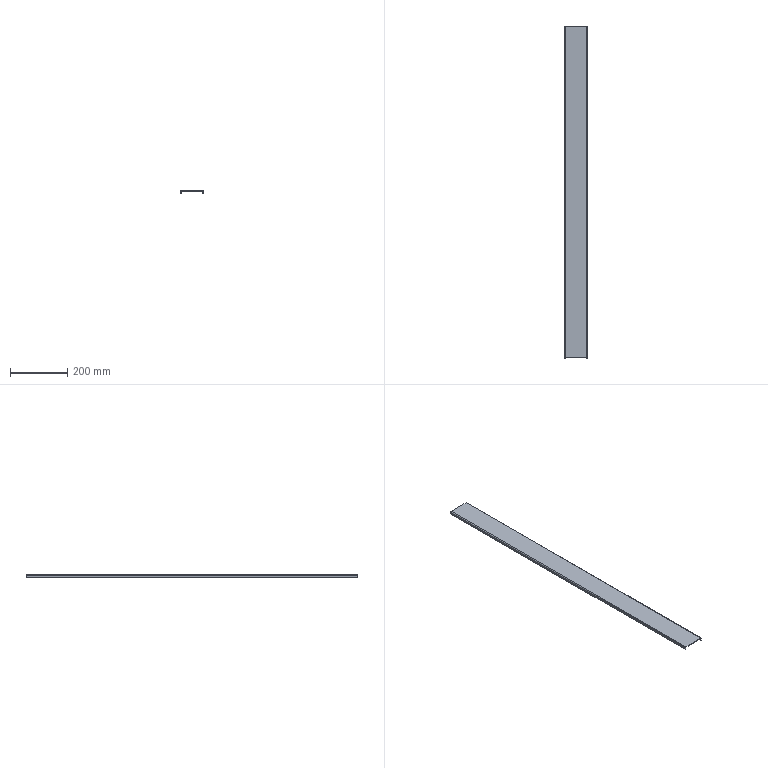Part | SolidWorks | features BaseBody 1 | 1 solid | 22 faces | box 80 x 1161 x 10 mm | volume 271377 mm3 | plane 18 | cylinder 4 | commonest cylinder face diameters 1 x2 6 x2
STEP:
#1=CARTESIAN_POINT('',(-37.5,580.5,-10.));
#2=VERTEX_POINT('',#1);
#3=CARTESIAN_POINT('',(-37.5,-580.5,-10.));
#4=VERTEX_POINT('',#3);
#5=CARTESIAN_POINT('',(-37.5,-580.5,-10.));
#6=DIRECTION('',(0.,-1.,0.));
#7=VECTOR('',#6,1000.);
#8=LINE('',#5,#7);
#9=EDGE_CURVE('',#2,#4,#8,.T.);
#10=ORIENTED_EDGE('',*,*,#9,.T.);
#11=CARTESIAN_POINT('',(-40.,-580.5,-10.));
#12=VERTEX_POINT('',#11);
#13=CARTESIAN_POINT('',(-40.,-580.5,-10.));
#14=DIRECTION('',(1.,0.,0.));
#15=VECTOR('',#14,1000.);
#16=LINE('',#13,#15);
#17=EDGE_CURVE('',#12,#4,#16,.T.);
#18=ORIENTED_EDGE('',*,*,#17,.F.);
#19=CARTESIAN_POINT('',(-40.,580.5,-10.));
#20=VERTEX_POINT('',#19);
#21=CARTESIAN_POINT('',(-40.,0.,-10.));
#22=DIRECTION('',(0.,-1.,0.));
#23=VECTOR('',#22,1000.);
#24=LINE('',#21,#23);
#25=EDGE_CURVE('',#20,#12,#24,.T.);
#26=ORIENTED_EDGE('',*,*,#25,.F.);
#27=CARTESIAN_POINT('',(-40.,580.5,-10.));
#28=DIRECTION('',(1.,0.,0.));
#29=VECTOR('',#28,1000.);
#30=LINE('',#27,#29);
#31=EDGE_CURVE('',#20,#2,#30,.T.);
#32=ORIENTED_EDGE('',*,*,#31,.T.);
#33=EDGE_LOOP('',(#10,#18,#26,#32));
#34=FACE_OUTER_BOUND('',#33,.T.);
#35=CARTESIAN_POINT('',(-40.,-580.5,-10.));
#36=DIRECTION('',(0.,0.,1.));
#37=DIRECTION('',(1.,0.,0.));
#38=AXIS2_PLACEMENT_3D('',#35,#36,#37);
#39=PLANE('',#38);
#40=ADVANCED_FACE('',(#34),#39,.F.);
#41=CARTESIAN_POINT('',(-37.5,580.5,-3.));
#42=VERTEX_POINT('',#41);
#43=CARTESIAN_POINT('',(-37.5,580.5,-10.));
#44=DIRECTION('',(0.,0.,-1.));
#45=VECTOR('',#44,1000.);
#46=LINE('',#43,#45);
#47=EDGE_CURVE('',#42,#2,#46,.T.);
#48=ORIENTED_EDGE('',*,*,#47,.F.);
#49=CARTESIAN_POINT('',(-37.5,-580.5,-3.));
#50=VERTEX_POINT('',#49);
#51=CARTESIAN_POINT('',(-37.5,-580.5,-3.));
#52=DIRECTION('',(0.,1.,0.));
#53=VECTOR('',#52,1000.);
#54=LINE('',#51,#53);
#55=EDGE_CURVE('',#50,#42,#54,.T.);
#56=ORIENTED_EDGE('',*,*,#55,.F.);
#57=CARTESIAN_POINT('',(-37.5,-580.5,-2.5));
#58=DIRECTION('',(0.,0.,1.));
#59=VECTOR('',#58,1000.);
#60=LINE('',#57,#59);
#61=EDGE_CURVE('',#4,#50,#60,.T.);
#62=ORIENTED_EDGE('',*,*,#61,.F.);
#63=ORIENTED_EDGE('',*,*,#9,.F.);
#64=EDGE_LOOP('',(#48,#56,#62,#63));
#65=FACE_OUTER_BOUND('',#64,.T.);
#66=CARTESIAN_POINT('',(-37.5,0.,0.));
#67=DIRECTION('',(1.,0.,0.));
#68=DIRECTION('',(0.,0.,-1.));
#69=AXIS2_PLACEMENT_3D('',#66,#67,#68);
#70=PLANE('',#69);
#71=ADVANCED_FACE('',(#65),#70,.T.);
#72=CARTESIAN_POINT('',(-40.,580.5,-3.));
#73=VERTEX_POINT('',#72);
#74=CARTESIAN_POINT('',(-40.,-580.5,-3.));
#75=VERTEX_POINT('',#74);
#76=CARTESIAN_POINT('',(-40.,-580.5,-3.));
#77=DIRECTION('',(0.,-1.,0.));
#78=VECTOR('',#77,1000.);
#79=LINE('',#76,#78);
#80=EDGE_CURVE('',#73,#75,#79,.T.);
#81=ORIENTED_EDGE('',*,*,#80,.F.);
#82=CARTESIAN_POINT('',(-40.,580.5,0.));
#83=DIRECTION('',(0.,0.,-1.));
#84=VECTOR('',#83,1000.);
#85=LINE('',#82,#84);
#86=EDGE_CURVE('',#73,#20,#85,.T.);
#87=ORIENTED_EDGE('',*,*,#86,.T.);
#88=ORIENTED_EDGE('',*,*,#25,.T.);
#89=CARTESIAN_POINT('',(-40.,-580.5,0.));
#90=DIRECTION('',(0.,0.,1.));
#91=VECTOR('',#90,1000.);
#92=LINE('',#89,#91);
#93=EDGE_CURVE('',#12,#75,#92,.T.);
#94=ORIENTED_EDGE('',*,*,#93,.T.);
#95=EDGE_LOOP('',(#81,#87,#88,#94));
#96=FACE_OUTER_BOUND('',#95,.T.);
#97=CARTESIAN_POINT('',(-40.,0.,0.));
#98=DIRECTION('',(1.,0.,0.));
#99=DIRECTION('',(0.,0.,-1.));
#100=AXIS2_PLACEMENT_3D('',#97,#98,#99);
#101=PLANE('',#100);
#102=ADVANCED_FACE('',(#96),#101,.F.);
#103=CARTESIAN_POINT('',(-40.,-580.5,-3.));
#104=DIRECTION('',(-1.,0.,0.));
#105=VECTOR('',#104,1000.);
#106=LINE('',#103,#105);
#107=EDGE_CURVE('',#50,#75,#106,.T.);
#108=ORIENTED_EDGE('',*,*,#107,.T.);
#109=ORIENTED_EDGE('',*,*,#93,.F.);
#110=ORIENTED_EDGE('',*,*,#17,.T.);
#111=ORIENTED_EDGE('',*,*,#61,.T.);
#112=EDGE_LOOP('',(#108,#109,#110,#111));
#113=FACE_OUTER_BOUND('',#112,.T.);
#114=CARTESIAN_POINT('',(-40.,-580.5,-2.5));
#115=DIRECTION('',(0.,1.,0.));
#116=DIRECTION('',(1.,0.,0.));
#117=AXIS2_PLACEMENT_3D('',#114,#115,#116);
#118=PLANE('',#117);
#119=ADVANCED_FACE('',(#113),#118,.F.);
#120=CARTESIAN_POINT('',(-37.5,580.5,-3.));
#121=DIRECTION('',(-1.,0.,0.));
#122=VECTOR('',#121,1000.);
#123=LINE('',#120,#122);
#124=EDGE_CURVE('',#42,#73,#123,.T.);
#125=ORIENTED_EDGE('',*,*,#124,.F.);
#126=ORIENTED_EDGE('',*,*,#47,.T.);
#127=ORIENTED_EDGE('',*,*,#31,.F.);
#128=ORIENTED_EDGE('',*,*,#86,.F.);
#129=EDGE_LOOP('',(#125,#126,#127,#128));
#130=FACE_OUTER_BOUND('',#129,.T.);
#131=CARTESIAN_POINT('',(-40.,580.5,-10.));
#132=DIRECTION('',(0.,-1.,0.));
#133=DIRECTION('',(0.,0.,-1.));
#134=AXIS2_PLACEMENT_3D('',#131,#132,#133);
#135=PLANE('',#134);
#136=ADVANCED_FACE('',(#130),#135,.F.);
#137=CARTESIAN_POINT('',(-37.,580.5,-2.5));
#138=VERTEX_POINT('',#137);
#139=CARTESIAN_POINT('',(-37.,-580.5,-2.5));
#140=VERTEX_POINT('',#139);
#141=CARTESIAN_POINT('',(-37.,580.5,-2.5));
#142=DIRECTION('',(0.,-1.,0.));
#143=VECTOR('',#142,1000.);
#144=LINE('',#141,#143);
#145=EDGE_CURVE('',#138,#140,#144,.T.);
#146=ORIENTED_EDGE('',*,*,#145,.T.);
#147=CARTESIAN_POINT('',(-37.,-580.5,-3.));
#148=DIRECTION('',(0.,-1.,0.));
#149=DIRECTION('',(0.,0.,1.));
#150=AXIS2_PLACEMENT_3D('',#147,#148,#149);
#151=CIRCLE('',#150,0.5);
#152=EDGE_CURVE('',#140,#50,#151,.T.);
#153=ORIENTED_EDGE('',*,*,#152,.T.);
#154=ORIENTED_EDGE('',*,*,#55,.T.);
#155=CARTESIAN_POINT('',(-37.,580.5,-3.));
#156=DIRECTION('',(0.,1.,0.));
#157=DIRECTION('',(0.,0.,1.));
#158=AXIS2_PLACEMENT_3D('',#155,#156,#157);
#159=CIRCLE('',#158,0.5);
#160=EDGE_CURVE('',#42,#138,#159,.T.);
#161=ORIENTED_EDGE('',*,*,#160,.T.);
#162=EDGE_LOOP('',(#146,#153,#154,#161));
#163=FACE_OUTER_BOUND('',#162,.T.);
#164=CARTESIAN_POINT('',(-37.,580.5,-3.));
#165=DIRECTION('',(0.,1.,0.));
#166=DIRECTION('',(-1.,0.,0.));
#167=AXIS2_PLACEMENT_3D('',#164,#165,#166);
#168=CYLINDRICAL_SURFACE('',#167,0.5);
#169=ADVANCED_FACE('',(#163),#168,.F.);
#170=CARTESIAN_POINT('',(-37.,580.5,0.));
#171=VERTEX_POINT('',#170);
#172=CARTESIAN_POINT('',(-37.,-580.5,0.));
#173=VERTEX_POINT('',#172);
#174=CARTESIAN_POINT('',(-37.,580.5,0.));
#175=DIRECTION('',(0.,-1.,0.));
#176=VECTOR('',#175,1000.);
#177=LINE('',#174,#176);
#178=EDGE_CURVE('',#171,#173,#177,.T.);
#179=ORIENTED_EDGE('',*,*,#178,.F.);
#180=CARTESIAN_POINT('',(-37.,580.5,-3.));
#181=DIRECTION('',(0.,1.,0.));
#182=DIRECTION('',(0.,0.,1.));
#183=AXIS2_PLACEMENT_3D('',#180,#181,#182);
#184=CIRCLE('',#183,3.);
#185=EDGE_CURVE('',#73,#171,#184,.T.);
#186=ORIENTED_EDGE('',*,*,#185,.F.);
#187=ORIENTED_EDGE('',*,*,#80,.T.);
#188=CARTESIAN_POINT('',(-37.,-580.5,-3.));
#189=DIRECTION('',(0.,-1.,0.));
#190=DIRECTION('',(0.,0.,1.));
#191=AXIS2_PLACEMENT_3D('',#188,#189,#190);
#192=CIRCLE('',#191,3.);
#193=EDGE_CURVE('',#173,#75,#192,.T.);
#194=ORIENTED_EDGE('',*,*,#193,.F.);
#195=EDGE_LOOP('',(#179,#186,#187,#194));
#196=FACE_OUTER_BOUND('',#195,.T.);
#197=CARTESIAN_POINT('',(-37.,580.5,-3.));
#198=DIRECTION('',(0.,1.,0.));
#199=DIRECTION('',(-1.,0.,0.));
#200=AXIS2_PLACEMENT_3D('',#197,#198,#199);
#201=CYLINDRICAL_SURFACE('',#200,3.);
#202=ADVANCED_FACE('',(#196),#201,.T.);
#203=ORIENTED_EDGE('',*,*,#160,.F.);
#204=ORIENTED_EDGE('',*,*,#124,.T.);
#205=ORIENTED_EDGE('',*,*,#185,.T.);
#206=CARTESIAN_POINT('',(-37.,580.5,-2.5));
#207=DIRECTION('',(0.,0.,1.));
#208=VECTOR('',#207,1000.);
#209=LINE('',#206,#208);
#210=EDGE_CURVE('',#138,#171,#209,.T.);
#211=ORIENTED_EDGE('',*,*,#210,.F.);
#212=EDGE_LOOP('',(#203,#204,#205,#211));
#213=FACE_OUTER_BOUND('',#212,.T.);
#214=CARTESIAN_POINT('',(-37.,580.5,-3.));
#215=DIRECTION('',(0.,-1.,0.));
#216=DIRECTION('',(0.,0.,-1.));
#217=AXIS2_PLACEMENT_3D('',#214,#215,#216);
#218=PLANE('',#217);
#219=ADVANCED_FACE('',(#213),#218,.F.);
#220=ORIENTED_EDGE('',*,*,#107,.F.);
#221=ORIENTED_EDGE('',*,*,#152,.F.);
#222=CARTESIAN_POINT('',(-37.,-580.5,-2.5));
#223=DIRECTION('',(0.,0.,1.));
#224=VECTOR('',#223,1000.);
#225=LINE('',#222,#224);
#226=EDGE_CURVE('',#140,#173,#225,.T.);
#227=ORIENTED_EDGE('',*,*,#226,.T.);
#228=ORIENTED_EDGE('',*,*,#193,.T.);
#229=EDGE_LOOP('',(#220,#221,#227,#228));
#230=FACE_OUTER_BOUND('',#229,.T.);
#231=CARTESIAN_POINT('',(-37.,-580.5,-3.));
#232=DIRECTION('',(0.,-1.,0.));
#233=DIRECTION('',(0.,0.,-1.));
#234=AXIS2_PLACEMENT_3D('',#231,#232,#233);
#235=PLANE('',#234);
#236=ADVANCED_FACE('',(#230),#235,.T.);
#237=CARTESIAN_POINT('',(37.5,-580.5,-10.));
#238=VERTEX_POINT('',#237);
#239=CARTESIAN_POINT('',(37.5,580.5,-10.));
#240=VERTEX_POINT('',#239);
#241=CARTESIAN_POINT('',(37.5,580.5,-10.));
#242=DIRECTION('',(0.,1.,0.));
#243=VECTOR('',#242,1000.);
#244=LINE('',#241,#243);
#245=EDGE_CURVE('',#238,#240,#244,.T.);
#246=ORIENTED_EDGE('',*,*,#245,.T.);
#247=CARTESIAN_POINT('',(40.,580.5,-10.));
#248=VERTEX_POINT('',#247);
#249=CARTESIAN_POINT('',(40.,580.5,-10.));
#250=DIRECTION('',(-1.,0.,0.));
#251=VECTOR('',#250,1000.);
#252=LINE('',#249,#251);
#253=EDGE_CURVE('',#248,#240,#252,.T.);
#254=ORIENTED_EDGE('',*,*,#253,.F.);
#255=CARTESIAN_POINT('',(40.,-580.5,-10.));
#256=VERTEX_POINT('',#255);
#257=CARTESIAN_POINT('',(40.,0.,-10.));
#258=DIRECTION('',(0.,1.,0.));
#259=VECTOR('',#258,1000.);
#260=LINE('',#257,#259);
#261=EDGE_CURVE('',#256,#248,#260,.T.);
#262=ORIENTED_EDGE('',*,*,#261,.F.);
#263=CARTESIAN_POINT('',(40.,-580.5,-10.));
#264=DIRECTION('',(-1.,0.,0.));
#265=VECTOR('',#264,1000.);
#266=LINE('',#263,#265);
#267=EDGE_CURVE('',#256,#238,#266,.T.);
#268=ORIENTED_EDGE('',*,*,#267,.T.);
#269=EDGE_LOOP('',(#246,#254,#262,#268));
#270=FACE_OUTER_BOUND('',#269,.T.);
#271=CARTESIAN_POINT('',(40.,580.5,-10.));
#272=DIRECTION('',(0.,0.,1.));
#273=DIRECTION('',(1.,0.,0.));
#274=AXIS2_PLACEMENT_3D('',#271,#272,#273);
#275=PLANE('',#274);
#276=ADVANCED_FACE('',(#270),#275,.F.);
#277=CARTESIAN_POINT('',(37.5,-580.5,-3.));
#278=VERTEX_POINT('',#277);
#279=CARTESIAN_POINT('',(37.5,-580.5,-10.));
#280=DIRECTION('',(0.,0.,-1.));
#281=VECTOR('',#280,1000.);
#282=LINE('',#279,#281);
#283=EDGE_CURVE('',#278,#238,#282,.T.);
#284=ORIENTED_EDGE('',*,*,#283,.F.);
#285=CARTESIAN_POINT('',(37.5,580.5,-3.));
#286=VERTEX_POINT('',#285);
#287=CARTESIAN_POINT('',(37.5,580.5,-3.));
#288=DIRECTION('',(0.,-1.,0.));
#289=VECTOR('',#288,1000.);
#290=LINE('',#287,#289);
#291=EDGE_CURVE('',#286,#278,#290,.T.);
#292=ORIENTED_EDGE('',*,*,#291,.F.);
#293=CARTESIAN_POINT('',(37.5,580.5,-2.5));
#294=DIRECTION('',(0.,0.,1.));
#295=VECTOR('',#294,1000.);
#296=LINE('',#293,#295);
#297=EDGE_CURVE('',#240,#286,#296,.T.);
#298=ORIENTED_EDGE('',*,*,#297,.F.);
#299=ORIENTED_EDGE('',*,*,#245,.F.);
#300=EDGE_LOOP('',(#284,#292,#298,#299));
#301=FACE_OUTER_BOUND('',#300,.T.);
#302=CARTESIAN_POINT('',(37.5,0.,0.));
#303=DIRECTION('',(-1.,0.,0.));
#304=DIRECTION('',(0.,0.,1.));
#305=AXIS2_PLACEMENT_3D('',#302,#303,#304);
#306=PLANE('',#305);
#307=ADVANCED_FACE('',(#301),#306,.T.);
#308=CARTESIAN_POINT('',(40.,-580.5,-3.));
#309=VERTEX_POINT('',#308);
#310=CARTESIAN_POINT('',(40.,580.5,-3.));
#311=VERTEX_POINT('',#310);
#312=CARTESIAN_POINT('',(40.,580.5,-3.));
#313=DIRECTION('',(0.,1.,0.));
#314=VECTOR('',#313,1000.);
#315=LINE('',#312,#314);
#316=EDGE_CURVE('',#309,#311,#315,.T.);
#317=ORIENTED_EDGE('',*,*,#316,.F.);
#318=CARTESIAN_POINT('',(40.,-580.5,0.));
#319=DIRECTION('',(0.,0.,-1.));
#320=VECTOR('',#319,1000.);
#321=LINE('',#318,#320);
#322=EDGE_CURVE('',#309,#256,#321,.T.);
#323=ORIENTED_EDGE('',*,*,#322,.T.);
#324=ORIENTED_EDGE('',*,*,#261,.T.);
#325=CARTESIAN_POINT('',(40.,580.5,0.));
#326=DIRECTION('',(0.,0.,1.));
#327=VECTOR('',#326,1000.);
#328=LINE('',#325,#327);
#329=EDGE_CURVE('',#248,#311,#328,.T.);
#330=ORIENTED_EDGE('',*,*,#329,.T.);
#331=EDGE_LOOP('',(#317,#323,#324,#330));
#332=FACE_OUTER_BOUND('',#331,.T.);
#333=CARTESIAN_POINT('',(40.,0.,0.));
#334=DIRECTION('',(-1.,0.,0.));
#335=DIRECTION('',(0.,0.,1.));
#336=AXIS2_PLACEMENT_3D('',#333,#334,#335);
#337=PLANE('',#336);
#338=ADVANCED_FACE('',(#332),#337,.F.);
#339=CARTESIAN_POINT('',(40.,580.5,-3.));
#340=DIRECTION('',(1.,0.,0.));
#341=VECTOR('',#340,1000.);
#342=LINE('',#339,#341);
#343=EDGE_CURVE('',#286,#311,#342,.T.);
#344=ORIENTED_EDGE('',*,*,#343,.T.);
#345=ORIENTED_EDGE('',*,*,#329,.F.);
#346=ORIENTED_EDGE('',*,*,#253,.T.);
#347=ORIENTED_EDGE('',*,*,#297,.T.);
#348=EDGE_LOOP('',(#344,#345,#346,#347));
#349=FACE_OUTER_BOUND('',#348,.T.);
#350=CARTESIAN_POINT('',(40.,580.5,-2.5));
#351=DIRECTION('',(0.,-1.,0.));
#352=DIRECTION('',(0.,0.,-1.));
#353=AXIS2_PLACEMENT_3D('',#350,#351,#352);
#354=PLANE('',#353);
#355=ADVANCED_FACE('',(#349),#354,.F.);
#356=CARTESIAN_POINT('',(37.5,-580.5,-3.));
#357=DIRECTION('',(1.,0.,0.));
#358=VECTOR('',#357,1000.);
#359=LINE('',#356,#358);
#360=EDGE_CURVE('',#278,#309,#359,.T.);
#361=ORIENTED_EDGE('',*,*,#360,.F.);
#362=ORIENTED_EDGE('',*,*,#283,.T.);
#363=ORIENTED_EDGE('',*,*,#267,.F.);
#364=ORIENTED_EDGE('',*,*,#322,.F.);
#365=EDGE_LOOP('',(#361,#362,#363,#364));
#366=FACE_OUTER_BOUND('',#365,.T.);
#367=CARTESIAN_POINT('',(40.,-580.5,-10.));
#368=DIRECTION('',(0.,1.,0.));
#369=DIRECTION('',(1.,0.,0.));
#370=AXIS2_PLACEMENT_3D('',#367,#368,#369);
#371=PLANE('',#370);
#372=ADVANCED_FACE('',(#366),#371,.F.);
#373=CARTESIAN_POINT('',(37.,-580.5,-2.5));
#374=VERTEX_POINT('',#373);
#375=CARTESIAN_POINT('',(37.,580.5,-2.5));
#376=VERTEX_POINT('',#375);
#377=CARTESIAN_POINT('',(37.,-580.5,-2.5));
#378=DIRECTION('',(0.,1.,0.));
#379=VECTOR('',#378,1000.);
#380=LINE('',#377,#379);
#381=EDGE_CURVE('',#374,#376,#380,.T.);
#382=ORIENTED_EDGE('',*,*,#381,.T.);
#383=CARTESIAN_POINT('',(37.,580.5,-3.));
#384=DIRECTION('',(0.,1.,0.));
#385=DIRECTION('',(0.,0.,-1.));
#386=AXIS2_PLACEMENT_3D('',#383,#384,#385);
#387=CIRCLE('',#386,0.5);
#388=EDGE_CURVE('',#376,#286,#387,.T.);
#389=ORIENTED_EDGE('',*,*,#388,.T.);
#390=ORIENTED_EDGE('',*,*,#291,.T.);
#391=CARTESIAN_POINT('',(37.,-580.5,-3.));
#392=DIRECTION('',(0.,-1.,0.));
#393=DIRECTION('',(0.,0.,-1.));
#394=AXIS2_PLACEMENT_3D('',#391,#392,#393);
#395=CIRCLE('',#394,0.5);
#396=EDGE_CURVE('',#278,#374,#395,.T.);
#397=ORIENTED_EDGE('',*,*,#396,.T.);
#398=EDGE_LOOP('',(#382,#389,#390,#397));
#399=FACE_OUTER_BOUND('',#398,.T.);
#400=CARTESIAN_POINT('',(37.,-580.5,-3.));
#401=DIRECTION('',(0.,-1.,0.));
#402=DIRECTION('',(1.,0.,0.));
#403=AXIS2_PLACEMENT_3D('',#400,#401,#402);
#404=CYLINDRICAL_SURFACE('',#403,0.5);
#405=ADVANCED_FACE('',(#399),#404,.F.);
#406=CARTESIAN_POINT('',(37.,-580.5,0.));
#407=VERTEX_POINT('',#406);
#408=CARTESIAN_POINT('',(37.,580.5,0.));
#409=VERTEX_POINT('',#408);
#410=CARTESIAN_POINT('',(37.,-580.5,0.));
#411=DIRECTION('',(0.,1.,0.));
#412=VECTOR('',#411,1000.);
#413=LINE('',#410,#412);
#414=EDGE_CURVE('',#407,#409,#413,.T.);
#415=ORIENTED_EDGE('',*,*,#414,.F.);
#416=CARTESIAN_POINT('',(37.,-580.5,-3.));
#417=DIRECTION('',(0.,-1.,0.));
#418=DIRECTION('',(0.,0.,-1.));
#419=AXIS2_PLACEMENT_3D('',#416,#417,#418);
#420=CIRCLE('',#419,3.);
#421=EDGE_CURVE('',#309,#407,#420,.T.);
#422=ORIENTED_EDGE('',*,*,#421,.F.);
#423=ORIENTED_EDGE('',*,*,#316,.T.);
#424=CARTESIAN_POINT('',(37.,580.5,-3.));
#425=DIRECTION('',(0.,1.,0.));
#426=DIRECTION('',(0.,0.,-1.));
#427=AXIS2_PLACEMENT_3D('',#424,#425,#426);
#428=CIRCLE('',#427,3.);
#429=EDGE_CURVE('',#409,#311,#428,.T.);
#430=ORIENTED_EDGE('',*,*,#429,.F.);
#431=EDGE_LOOP('',(#415,#422,#423,#430));
#432=FACE_OUTER_BOUND('',#431,.T.);
#433=CARTESIAN_POINT('',(37.,-580.5,-3.));
#434=DIRECTION('',(0.,-1.,0.));
#435=DIRECTION('',(1.,0.,0.));
#436=AXIS2_PLACEMENT_3D('',#433,#434,#435);
#437=CYLINDRICAL_SURFACE('',#436,3.);
#438=ADVANCED_FACE('',(#432),#437,.T.);
#439=ORIENTED_EDGE('',*,*,#396,.F.);
#440=ORIENTED_EDGE('',*,*,#360,.T.);
#441=ORIENTED_EDGE('',*,*,#421,.T.);
#442=CARTESIAN_POINT('',(37.,-580.5,-2.5));
#443=DIRECTION('',(0.,0.,1.));
#444=VECTOR('',#443,1000.);
#445=LINE('',#442,#444);
#446=EDGE_CURVE('',#374,#407,#445,.T.);
#447=ORIENTED_EDGE('',*,*,#446,.F.);
#448=EDGE_LOOP('',(#439,#440,#441,#447));
#449=FACE_OUTER_BOUND('',#448,.T.);
#450=CARTESIAN_POINT('',(37.,-580.5,-3.));
#451=DIRECTION('',(0.,1.,0.));
#452=DIRECTION('',(1.,0.,0.));
#453=AXIS2_PLACEMENT_3D('',#450,#451,#452);
#454=PLANE('',#453);
#455=ADVANCED_FACE('',(#449),#454,.F.);
#456=ORIENTED_EDGE('',*,*,#343,.F.);
#457=ORIENTED_EDGE('',*,*,#388,.F.);
#458=CARTESIAN_POINT('',(37.,580.5,-2.5));
#459=DIRECTION('',(0.,0.,1.));
#460=VECTOR('',#459,1000.);
#461=LINE('',#458,#460);
#462=EDGE_CURVE('',#376,#409,#461,.T.);
#463=ORIENTED_EDGE('',*,*,#462,.T.);
#464=ORIENTED_EDGE('',*,*,#429,.T.);
#465=EDGE_LOOP('',(#456,#457,#463,#464));
#466=FACE_OUTER_BOUND('',#465,.T.);
#467=CARTESIAN_POINT('',(37.,580.5,-3.));
#468=DIRECTION('',(0.,1.,0.));
#469=DIRECTION('',(1.,0.,0.));
#470=AXIS2_PLACEMENT_3D('',#467,#468,#469);
#471=PLANE('',#470);
#472=ADVANCED_FACE('',(#466),#471,.T.);
#473=ORIENTED_EDGE('',*,*,#226,.F.);
#474=CARTESIAN_POINT('',(40.,-580.5,-2.5));
#475=DIRECTION('',(1.,0.,0.));
#476=VECTOR('',#475,1000.);
#477=LINE('',#474,#476);
#478=EDGE_CURVE('',#140,#374,#477,.T.);
#479=ORIENTED_EDGE('',*,*,#478,.T.);
#480=ORIENTED_EDGE('',*,*,#446,.T.);
#481=CARTESIAN_POINT('',(40.,-580.5,0.));
#482=DIRECTION('',(1.,0.,0.));
#483=VECTOR('',#482,1000.);
#484=LINE('',#481,#483);
#485=EDGE_CURVE('',#173,#407,#484,.T.);
#486=ORIENTED_EDGE('',*,*,#485,.F.);
#487=EDGE_LOOP('',(#473,#479,#480,#486));
#488=FACE_OUTER_BOUND('',#487,.T.);
#489=CARTESIAN_POINT('',(40.,-580.5,-2.5));
#490=DIRECTION('',(0.,-1.,0.));
#491=DIRECTION('',(0.,0.,-1.));
#492=AXIS2_PLACEMENT_3D('',#489,#490,#491);
#493=PLANE('',#492);
#494=ADVANCED_FACE('',(#488),#493,.T.);
#495=CARTESIAN_POINT('',(40.,580.5,-2.5));
#496=DIRECTION('',(-1.,0.,0.));
#497=VECTOR('',#496,1000.);
#498=LINE('',#495,#497);
#499=EDGE_CURVE('',#376,#138,#498,.T.);
#500=ORIENTED_EDGE('',*,*,#499,.T.);
#501=ORIENTED_EDGE('',*,*,#210,.T.);
#502=CARTESIAN_POINT('',(40.,580.5,0.));
#503=DIRECTION('',(-1.,0.,0.));
#504=VECTOR('',#503,1000.);
#505=LINE('',#502,#504);
#506=EDGE_CURVE('',#409,#171,#505,.T.);
#507=ORIENTED_EDGE('',*,*,#506,.F.);
#508=ORIENTED_EDGE('',*,*,#462,.F.);
#509=EDGE_LOOP('',(#500,#501,#507,#508));
#510=FACE_OUTER_BOUND('',#509,.T.);
#511=CARTESIAN_POINT('',(40.,580.5,-2.5));
#512=DIRECTION('',(0.,1.,0.));
#513=DIRECTION('',(1.,0.,0.));
#514=AXIS2_PLACEMENT_3D('',#511,#512,#513);
#515=PLANE('',#514);
#516=ADVANCED_FACE('',(#510),#515,.T.);
#517=ORIENTED_EDGE('',*,*,#178,.T.);
#518=ORIENTED_EDGE('',*,*,#485,.T.);
#519=ORIENTED_EDGE('',*,*,#414,.T.);
#520=ORIENTED_EDGE('',*,*,#506,.T.);
#521=EDGE_LOOP('',(#517,#518,#519,#520));
#522=FACE_OUTER_BOUND('',#521,.T.);
#523=CARTESIAN_POINT('',(0.,0.,0.));
#524=DIRECTION('',(0.,0.,-1.));
#525=DIRECTION('',(0.,-1.,0.));
#526=AXIS2_PLACEMENT_3D('',#523,#524,#525);
#527=PLANE('',#526);
#528=ADVANCED_FACE('',(#522),#527,.F.);
#529=ORIENTED_EDGE('',*,*,#478,.F.);
#530=ORIENTED_EDGE('',*,*,#145,.F.);
#531=ORIENTED_EDGE('',*,*,#499,.F.);
#532=ORIENTED_EDGE('',*,*,#381,.F.);
#533=EDGE_LOOP('',(#529,#530,#531,#532));
#534=FACE_OUTER_BOUND('',#533,.T.);
#535=CARTESIAN_POINT('',(0.,0.,-2.5));
#536=DIRECTION('',(0.,0.,-1.));
#537=DIRECTION('',(0.,-1.,0.));
#538=AXIS2_PLACEMENT_3D('',#535,#536,#537);
#539=PLANE('',#538);
#540=ADVANCED_FACE('',(#534),#539,.T.);
#541=CLOSED_SHELL('',(#40,#71,#102,#119,#136,#169,#202,#219,#236,#276,#307,#338,#355,#372,#405,#438,#455,#472,#494,#516,#528,#540));
#542=MANIFOLD_SOLID_BREP('',#541);
#543=CARTESIAN_POINT('',(0.,0.,0.));
#544=DIRECTION('',(0.,0.,1.));
#545=DIRECTION('',(1.,0.,0.));
#546=AXIS2_PLACEMENT_3D('',#543,#544,#545);
#547=(LENGTH_UNIT()NAMED_UNIT(*)SI_UNIT(.MILLI.,.METRE.));
#548=UNCERTAINTY_MEASURE_WITH_UNIT(LENGTH_MEASURE(0.00001),#547,'','');
#549=(NAMED_UNIT(*)PLANE_ANGLE_UNIT()SI_UNIT($,.RADIAN.));
#550=(NAMED_UNIT(*)SI_UNIT($,.STERADIAN.)SOLID_ANGLE_UNIT());
#551=(GEOMETRIC_REPRESENTATION_CONTEXT(3)GLOBAL_UNCERTAINTY_ASSIGNED_CONTEXT((#548))GLOBAL_UNIT_ASSIGNED_CONTEXT((#547,#549,#550))REPRESENTATION_CONTEXT('',''));
#552=ADVANCED_BREP_SHAPE_REPRESENTATION('',(#542,#546),#551);